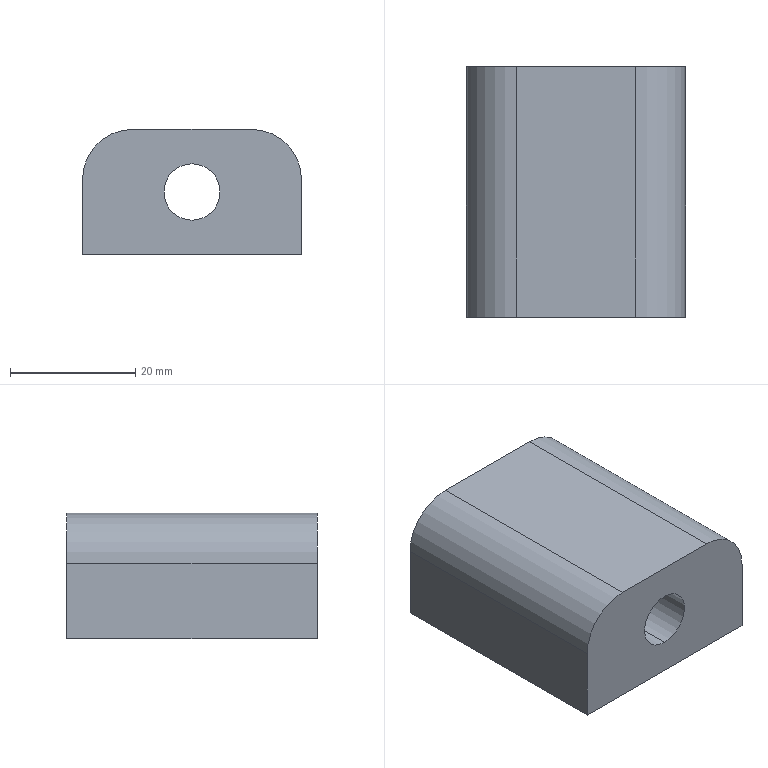Part | STEP file | 1 solid | 13 faces | box 35 x 40 x 20 mm | volume 23544 mm3 | plane 7 | cylinder 6 | commonest cylinder face diameters 9 x2 14 x2 16 x2
STEP:
#1=CARTESIAN_POINT('',(0.,0.,0.));
#2=DIRECTION('',(0.,0.,1.));
#3=DIRECTION('',(1.,0.,0.));
#4=AXIS2_PLACEMENT_3D('',#1,#2,#3);
#5=CARTESIAN_POINT('',(-72.862,-30.,211.03));
#6=VERTEX_POINT('',#5);
#7=CARTESIAN_POINT('',(-72.862,-39.,211.03));
#8=VERTEX_POINT('',#7);
#9=CARTESIAN_POINT('',(-72.862,-30.,211.03));
#10=DIRECTION('',(0.,-1.,0.));
#11=VECTOR('',#10,1.);
#12=LINE('',#9,#11);
#13=CARTESIAN_POINT('',(-72.862,-30.,218.03));
#14=DIRECTION('',(0.,-1.,0.));
#15=DIRECTION('',(0.,0.,-1.));
#16=AXIS2_PLACEMENT_3D('',#13,#14,#15);
#17=CYLINDRICAL_SURFACE('',#16,7.);
#18=CARTESIAN_POINT('',(6.283,0.));
#19=DIRECTION('',(0.,1.));
#20=VECTOR('',#19,1.);
#21=LINE('',#18,#20);
#22=(GEOMETRIC_REPRESENTATION_CONTEXT(2)PARAMETRIC_REPRESENTATION_CONTEXT()REPRESENTATION_CONTEXT('',''));
#23=DEFINITIONAL_REPRESENTATION('',(#21),#22);
#24=PCURVE('',#17,#23);
#25=CARTESIAN_POINT('',(-72.862,-30.,218.03));
#26=DIRECTION('',(0.,-1.,0.));
#27=DIRECTION('',(0.,0.,-1.));
#28=AXIS2_PLACEMENT_3D('',#25,#26,#27);
#29=CYLINDRICAL_SURFACE('',#28,7.);
#30=CARTESIAN_POINT('',(0.,0.));
#31=DIRECTION('',(0.,1.));
#32=VECTOR('',#31,1.);
#33=LINE('',#30,#32);
#34=(GEOMETRIC_REPRESENTATION_CONTEXT(2)PARAMETRIC_REPRESENTATION_CONTEXT()REPRESENTATION_CONTEXT('',''));
#35=DEFINITIONAL_REPRESENTATION('',(#33),#34);
#36=PCURVE('',#29,#35);
#37=SURFACE_CURVE('',#12,(#24,#36),.PCURVE_S1.);
#38=EDGE_CURVE('',#6,#8,#37,.T.);
#39=ORIENTED_EDGE('',*,*,#38,.T.);
#40=CARTESIAN_POINT('',(-72.862,-39.,225.03));
#41=VERTEX_POINT('',#40);
#42=CARTESIAN_POINT('',(-72.862,-39.,218.03));
#43=DIRECTION('',(0.,1.,0.));
#44=DIRECTION('',(0.,0.,1.));
#45=AXIS2_PLACEMENT_3D('',#42,#43,#44);
#46=CIRCLE('',#45,7.);
#47=CARTESIAN_POINT('',(9.425,9.));
#48=DIRECTION('',(-1.,0.));
#49=VECTOR('',#48,1.);
#50=LINE('',#47,#49);
#51=(GEOMETRIC_REPRESENTATION_CONTEXT(2)PARAMETRIC_REPRESENTATION_CONTEXT()REPRESENTATION_CONTEXT('',''));
#52=DEFINITIONAL_REPRESENTATION('',(#50),#51);
#53=PCURVE('',#17,#52);
#54=CARTESIAN_POINT('',(-72.862,-39.,218.03));
#55=DIRECTION('',(0.,-1.,0.));
#56=DIRECTION('',(0.,0.,-1.));
#57=AXIS2_PLACEMENT_3D('',#54,#55,#56);
#58=PLANE('',#57);
#59=CARTESIAN_POINT('',(-7.,0.));
#60=CARTESIAN_POINT('',(-7.,12.124));
#61=CARTESIAN_POINT('',(3.5,6.062));
#62=CARTESIAN_POINT('',(14.,0.));
#63=CARTESIAN_POINT('',(3.5,-6.062));
#64=CARTESIAN_POINT('',(-7.,-12.124));
#65=CARTESIAN_POINT('',(-7.,0.));
#66=(BOUNDED_CURVE()B_SPLINE_CURVE(2,(#59,#60,#61,#62,#63,#64,#65),.UNSPECIFIED.,.T.,.F.)B_SPLINE_CURVE_WITH_KNOTS((1,2,2,2,2,1),(-2.094,0.,2.094,4.189,6.283,8.378),.UNSPECIFIED.)CURVE()GEOMETRIC_REPRESENTATION_ITEM()RATIONAL_B_SPLINE_CURVE((1.,0.5,1.,0.5,1.,0.5,1.))REPRESENTATION_ITEM(''));
#67=(GEOMETRIC_REPRESENTATION_CONTEXT(2)PARAMETRIC_REPRESENTATION_CONTEXT()REPRESENTATION_CONTEXT('',''));
#68=DEFINITIONAL_REPRESENTATION('',(#66),#67);
#69=PCURVE('',#58,#68);
#70=SURFACE_CURVE('',#46,(#53,#69),.PCURVE_S1.);
#71=EDGE_CURVE('',#8,#41,#70,.T.);
#72=ORIENTED_EDGE('',*,*,#71,.T.);
#73=CARTESIAN_POINT('',(-72.862,-30.,225.03));
#74=VERTEX_POINT('',#73);
#75=CARTESIAN_POINT('',(-72.862,-30.,225.03));
#76=DIRECTION('',(0.,-1.,0.));
#77=VECTOR('',#76,1.);
#78=LINE('',#75,#77);
#79=CARTESIAN_POINT('',(3.142,0.));
#80=DIRECTION('',(0.,1.));
#81=VECTOR('',#80,1.);
#82=LINE('',#79,#81);
#83=(GEOMETRIC_REPRESENTATION_CONTEXT(2)PARAMETRIC_REPRESENTATION_CONTEXT()REPRESENTATION_CONTEXT('',''));
#84=DEFINITIONAL_REPRESENTATION('',(#82),#83);
#85=PCURVE('',#17,#84);
#86=CARTESIAN_POINT('',(3.142,0.));
#87=DIRECTION('',(0.,1.));
#88=VECTOR('',#87,1.);
#89=LINE('',#86,#88);
#90=(GEOMETRIC_REPRESENTATION_CONTEXT(2)PARAMETRIC_REPRESENTATION_CONTEXT()REPRESENTATION_CONTEXT('',''));
#91=DEFINITIONAL_REPRESENTATION('',(#89),#90);
#92=PCURVE('',#29,#91);
#93=SURFACE_CURVE('',#78,(#85,#92),.PCURVE_S1.);
#94=EDGE_CURVE('',#74,#41,#93,.T.);
#95=ORIENTED_EDGE('',*,*,#94,.F.);
#96=CARTESIAN_POINT('',(-72.862,-30.,218.03));
#97=DIRECTION('',(0.,-1.,0.));
#98=DIRECTION('',(0.,0.,-1.));
#99=AXIS2_PLACEMENT_3D('',#96,#97,#98);
#100=CIRCLE('',#99,7.);
#101=CARTESIAN_POINT('',(0.,0.));
#102=DIRECTION('',(1.,0.));
#103=VECTOR('',#102,1.);
#104=LINE('',#101,#103);
#105=(GEOMETRIC_REPRESENTATION_CONTEXT(2)PARAMETRIC_REPRESENTATION_CONTEXT()REPRESENTATION_CONTEXT('',''));
#106=DEFINITIONAL_REPRESENTATION('',(#104),#105);
#107=PCURVE('',#17,#106);
#108=CARTESIAN_POINT('',(-169.363,-30.,-22.97));
#109=DIRECTION('',(0.,1.,0.));
#110=DIRECTION('',(0.,0.,1.));
#111=AXIS2_PLACEMENT_3D('',#108,#109,#110);
#112=PLANE('',#111);
#113=CARTESIAN_POINT('',(234.,96.5));
#114=CARTESIAN_POINT('',(234.,108.624));
#115=CARTESIAN_POINT('',(244.5,102.562));
#116=CARTESIAN_POINT('',(255.,96.5));
#117=CARTESIAN_POINT('',(244.5,90.438));
#118=CARTESIAN_POINT('',(234.,84.376));
#119=CARTESIAN_POINT('',(234.,96.5));
#120=(BOUNDED_CURVE()B_SPLINE_CURVE(2,(#113,#114,#115,#116,#117,#118,#119),.UNSPECIFIED.,.T.,.F.)B_SPLINE_CURVE_WITH_KNOTS((1,2,2,2,2,1),(-2.094,0.,2.094,4.189,6.283,8.378),.UNSPECIFIED.)CURVE()GEOMETRIC_REPRESENTATION_ITEM()RATIONAL_B_SPLINE_CURVE((1.,0.5,1.,0.5,1.,0.5,1.))REPRESENTATION_ITEM(''));
#121=(GEOMETRIC_REPRESENTATION_CONTEXT(2)PARAMETRIC_REPRESENTATION_CONTEXT()REPRESENTATION_CONTEXT('',''));
#122=DEFINITIONAL_REPRESENTATION('',(#120),#121);
#123=PCURVE('',#112,#122);
#124=SURFACE_CURVE('',#100,(#107,#123),.PCURVE_S1.);
#125=EDGE_CURVE('',#74,#6,#124,.T.);
#126=ORIENTED_EDGE('',*,*,#125,.T.);
#127=EDGE_LOOP('',(#39,#72,#95,#126));
#128=FACE_BOUND('',#127,.F.);
#129=ADVANCED_FACE('',(#128),#17,.F.);
#130=CARTESIAN_POINT('',(-72.862,-39.,213.53));
#131=VERTEX_POINT('',#130);
#132=CARTESIAN_POINT('',(-72.862,-70.,213.53));
#133=VERTEX_POINT('',#132);
#134=CARTESIAN_POINT('',(-72.862,-30.,213.53));
#135=DIRECTION('',(0.,-1.,0.));
#136=VECTOR('',#135,1.);
#137=LINE('',#134,#136);
#138=CARTESIAN_POINT('',(-72.862,-30.,218.03));
#139=DIRECTION('',(0.,-1.,0.));
#140=DIRECTION('',(0.,0.,-1.));
#141=AXIS2_PLACEMENT_3D('',#138,#139,#140);
#142=CYLINDRICAL_SURFACE('',#141,4.5);
#143=CARTESIAN_POINT('',(6.283,0.));
#144=DIRECTION('',(0.,1.));
#145=VECTOR('',#144,1.);
#146=LINE('',#143,#145);
#147=(GEOMETRIC_REPRESENTATION_CONTEXT(2)PARAMETRIC_REPRESENTATION_CONTEXT()REPRESENTATION_CONTEXT('',''));
#148=DEFINITIONAL_REPRESENTATION('',(#146),#147);
#149=PCURVE('',#142,#148);
#150=CARTESIAN_POINT('',(-72.862,-30.,218.03));
#151=DIRECTION('',(0.,-1.,0.));
#152=DIRECTION('',(0.,0.,-1.));
#153=AXIS2_PLACEMENT_3D('',#150,#151,#152);
#154=CYLINDRICAL_SURFACE('',#153,4.5);
#155=CARTESIAN_POINT('',(0.,0.));
#156=DIRECTION('',(0.,1.));
#157=VECTOR('',#156,1.);
#158=LINE('',#155,#157);
#159=(GEOMETRIC_REPRESENTATION_CONTEXT(2)PARAMETRIC_REPRESENTATION_CONTEXT()REPRESENTATION_CONTEXT('',''));
#160=DEFINITIONAL_REPRESENTATION('',(#158),#159);
#161=PCURVE('',#154,#160);
#162=SURFACE_CURVE('',#137,(#149,#161),.PCURVE_S1.);
#163=EDGE_CURVE('',#131,#133,#162,.T.);
#164=ORIENTED_EDGE('',*,*,#163,.T.);
#165=CARTESIAN_POINT('',(-72.862,-70.,222.53));
#166=VERTEX_POINT('',#165);
#167=CARTESIAN_POINT('',(-72.862,-70.,218.03));
#168=DIRECTION('',(0.,1.,0.));
#169=DIRECTION('',(0.,0.,1.));
#170=AXIS2_PLACEMENT_3D('',#167,#168,#169);
#171=CIRCLE('',#170,4.5);
#172=CARTESIAN_POINT('',(9.425,40.));
#173=DIRECTION('',(-1.,0.));
#174=VECTOR('',#173,1.);
#175=LINE('',#172,#174);
#176=(GEOMETRIC_REPRESENTATION_CONTEXT(2)PARAMETRIC_REPRESENTATION_CONTEXT()REPRESENTATION_CONTEXT('',''));
#177=DEFINITIONAL_REPRESENTATION('',(#175),#176);
#178=PCURVE('',#142,#177);
#179=CARTESIAN_POINT('',(-72.862,-70.,23.556));
#180=DIRECTION('',(0.,-1.,0.));
#181=DIRECTION('',(0.,0.,-1.));
#182=AXIS2_PLACEMENT_3D('',#179,#180,#181);
#183=PLANE('',#182);
#184=CARTESIAN_POINT('',(-198.974,0.));
#185=CARTESIAN_POINT('',(-198.974,7.794));
#186=CARTESIAN_POINT('',(-192.224,3.897));
#187=CARTESIAN_POINT('',(-185.474,0.));
#188=CARTESIAN_POINT('',(-192.224,-3.897));
#189=CARTESIAN_POINT('',(-198.974,-7.794));
#190=CARTESIAN_POINT('',(-198.974,0.));
#191=(BOUNDED_CURVE()B_SPLINE_CURVE(2,(#184,#185,#186,#187,#188,#189,#190),.UNSPECIFIED.,.T.,.F.)B_SPLINE_CURVE_WITH_KNOTS((1,2,2,2,2,1),(-2.094,0.,2.094,4.189,6.283,8.378),.UNSPECIFIED.)CURVE()GEOMETRIC_REPRESENTATION_ITEM()RATIONAL_B_SPLINE_CURVE((1.,0.5,1.,0.5,1.,0.5,1.))REPRESENTATION_ITEM(''));
#192=(GEOMETRIC_REPRESENTATION_CONTEXT(2)PARAMETRIC_REPRESENTATION_CONTEXT()REPRESENTATION_CONTEXT('',''));
#193=DEFINITIONAL_REPRESENTATION('',(#191),#192);
#194=PCURVE('',#183,#193);
#195=SURFACE_CURVE('',#171,(#178,#194),.PCURVE_S1.);
#196=EDGE_CURVE('',#133,#166,#195,.T.);
#197=ORIENTED_EDGE('',*,*,#196,.T.);
#198=CARTESIAN_POINT('',(-72.862,-39.,222.53));
#199=VERTEX_POINT('',#198);
#200=CARTESIAN_POINT('',(-72.862,-30.,222.53));
#201=DIRECTION('',(0.,-1.,0.));
#202=VECTOR('',#201,1.);
#203=LINE('',#200,#202);
#204=CARTESIAN_POINT('',(3.142,0.));
#205=DIRECTION('',(0.,1.));
#206=VECTOR('',#205,1.);
#207=LINE('',#204,#206);
#208=(GEOMETRIC_REPRESENTATION_CONTEXT(2)PARAMETRIC_REPRESENTATION_CONTEXT()REPRESENTATION_CONTEXT('',''));
#209=DEFINITIONAL_REPRESENTATION('',(#207),#208);
#210=PCURVE('',#142,#209);
#211=CARTESIAN_POINT('',(3.142,0.));
#212=DIRECTION('',(0.,1.));
#213=VECTOR('',#212,1.);
#214=LINE('',#211,#213);
#215=(GEOMETRIC_REPRESENTATION_CONTEXT(2)PARAMETRIC_REPRESENTATION_CONTEXT()REPRESENTATION_CONTEXT('',''));
#216=DEFINITIONAL_REPRESENTATION('',(#214),#215);
#217=PCURVE('',#154,#216);
#218=SURFACE_CURVE('',#203,(#210,#217),.PCURVE_S1.);
#219=EDGE_CURVE('',#199,#166,#218,.T.);
#220=ORIENTED_EDGE('',*,*,#219,.F.);
#221=CARTESIAN_POINT('',(-72.862,-39.,218.03));
#222=DIRECTION('',(0.,1.,0.));
#223=DIRECTION('',(0.,0.,-1.));
#224=AXIS2_PLACEMENT_3D('',#221,#222,#223);
#225=CIRCLE('',#224,4.5);
#226=CARTESIAN_POINT('',(6.283,9.));
#227=DIRECTION('',(-1.,0.));
#228=VECTOR('',#227,1.);
#229=LINE('',#226,#228);
#230=(GEOMETRIC_REPRESENTATION_CONTEXT(2)PARAMETRIC_REPRESENTATION_CONTEXT()REPRESENTATION_CONTEXT('',''));
#231=DEFINITIONAL_REPRESENTATION('',(#229),#230);
#232=PCURVE('',#142,#231);
#233=CARTESIAN_POINT('',(4.5,0.));
#234=CARTESIAN_POINT('',(4.5,-7.794));
#235=CARTESIAN_POINT('',(-2.25,-3.897));
#236=CARTESIAN_POINT('',(-9.,0.));
#237=CARTESIAN_POINT('',(-2.25,3.897));
#238=CARTESIAN_POINT('',(4.5,7.794));
#239=CARTESIAN_POINT('',(4.5,0.));
#240=(BOUNDED_CURVE()B_SPLINE_CURVE(2,(#233,#234,#235,#236,#237,#238,#239),.UNSPECIFIED.,.T.,.F.)B_SPLINE_CURVE_WITH_KNOTS((1,2,2,2,2,1),(-2.094,0.,2.094,4.189,6.283,8.378),.UNSPECIFIED.)CURVE()GEOMETRIC_REPRESENTATION_ITEM()RATIONAL_B_SPLINE_CURVE((1.,0.5,1.,0.5,1.,0.5,1.))REPRESENTATION_ITEM(''));
#241=(GEOMETRIC_REPRESENTATION_CONTEXT(2)PARAMETRIC_REPRESENTATION_CONTEXT()REPRESENTATION_CONTEXT('',''));
#242=DEFINITIONAL_REPRESENTATION('',(#240),#241);
#243=PCURVE('',#58,#242);
#244=SURFACE_CURVE('',#225,(#232,#243),.PCURVE_S1.);
#245=EDGE_CURVE('',#131,#199,#244,.T.);
#246=ORIENTED_EDGE('',*,*,#245,.F.);
#247=EDGE_LOOP('',(#164,#197,#220,#246));
#248=FACE_BOUND('',#247,.F.);
#249=ADVANCED_FACE('',(#248),#142,.F.);
#250=CARTESIAN_POINT('',(-90.362,-70.,220.03));
#251=VERTEX_POINT('',#250);
#252=CARTESIAN_POINT('',(-82.362,-70.,228.03));
#253=VERTEX_POINT('',#252);
#254=CARTESIAN_POINT('',(-82.362,-70.,220.03));
#255=DIRECTION('',(0.,1.,0.));
#256=DIRECTION('',(0.,0.,-1.));
#257=AXIS2_PLACEMENT_3D('',#254,#255,#256);
#258=CIRCLE('',#257,8.);
#259=CARTESIAN_POINT('',(-188.474,-9.5));
#260=CARTESIAN_POINT('',(-188.474,-23.356));
#261=CARTESIAN_POINT('',(-200.474,-16.428));
#262=CARTESIAN_POINT('',(-212.474,-9.5));
#263=CARTESIAN_POINT('',(-200.474,-2.572));
#264=CARTESIAN_POINT('',(-188.474,4.356));
#265=CARTESIAN_POINT('',(-188.474,-9.5));
#266=(BOUNDED_CURVE()B_SPLINE_CURVE(2,(#259,#260,#261,#262,#263,#264,#265),.UNSPECIFIED.,.T.,.F.)B_SPLINE_CURVE_WITH_KNOTS((1,2,2,2,2,1),(-2.094,0.,2.094,4.189,6.283,8.378),.UNSPECIFIED.)CURVE()GEOMETRIC_REPRESENTATION_ITEM()RATIONAL_B_SPLINE_CURVE((1.,0.5,1.,0.5,1.,0.5,1.))REPRESENTATION_ITEM(''));
#267=(GEOMETRIC_REPRESENTATION_CONTEXT(2)PARAMETRIC_REPRESENTATION_CONTEXT()REPRESENTATION_CONTEXT('',''));
#268=DEFINITIONAL_REPRESENTATION('',(#266),#267);
#269=PCURVE('',#183,#268);
#270=CARTESIAN_POINT('',(-82.362,-85.,220.03));
#271=DIRECTION('',(0.,1.,0.));
#272=DIRECTION('',(0.,0.,1.));
#273=AXIS2_PLACEMENT_3D('',#270,#271,#272);
#274=CYLINDRICAL_SURFACE('',#273,8.);
#275=CARTESIAN_POINT('',(3.142,15.));
#276=DIRECTION('',(1.,0.));
#277=VECTOR('',#276,1.);
#278=LINE('',#275,#277);
#279=(GEOMETRIC_REPRESENTATION_CONTEXT(2)PARAMETRIC_REPRESENTATION_CONTEXT()REPRESENTATION_CONTEXT('',''));
#280=DEFINITIONAL_REPRESENTATION('',(#278),#279);
#281=PCURVE('',#274,#280);
#282=SURFACE_CURVE('',#258,(#269,#281),.PCURVE_S1.);
#283=EDGE_CURVE('',#251,#253,#282,.T.);
#284=ORIENTED_EDGE('',*,*,#283,.F.);
#285=CARTESIAN_POINT('',(-90.362,-70.,208.03));
#286=VERTEX_POINT('',#285);
#287=CARTESIAN_POINT('',(-90.362,-70.,155.78));
#288=DIRECTION('',(0.,0.,1.));
#289=VECTOR('',#288,1.);
#290=LINE('',#287,#289);
#291=CARTESIAN_POINT('',(-132.224,-17.5));
#292=DIRECTION('',(-1.,0.));
#293=VECTOR('',#292,1.);
#294=LINE('',#291,#293);
#295=(GEOMETRIC_REPRESENTATION_CONTEXT(2)PARAMETRIC_REPRESENTATION_CONTEXT()REPRESENTATION_CONTEXT('',''));
#296=DEFINITIONAL_REPRESENTATION('',(#294),#295);
#297=PCURVE('',#183,#296);
#298=CARTESIAN_POINT('',(-90.362,-85.,155.78));
#299=DIRECTION('',(-1.,0.,0.));
#300=DIRECTION('',(0.,0.,1.));
#301=AXIS2_PLACEMENT_3D('',#298,#299,#300);
#302=PLANE('',#301);
#303=CARTESIAN_POINT('',(0.,15.));
#304=DIRECTION('',(1.,0.));
#305=VECTOR('',#304,1.);
#306=LINE('',#303,#305);
#307=(GEOMETRIC_REPRESENTATION_CONTEXT(2)PARAMETRIC_REPRESENTATION_CONTEXT()REPRESENTATION_CONTEXT('',''));
#308=DEFINITIONAL_REPRESENTATION('',(#306),#307);
#309=PCURVE('',#302,#308);
#310=SURFACE_CURVE('',#290,(#297,#309),.PCURVE_S1.);
#311=EDGE_CURVE('',#286,#251,#310,.T.);
#312=ORIENTED_EDGE('',*,*,#311,.F.);
#313=CARTESIAN_POINT('',(-55.362,-70.,208.03));
#314=VERTEX_POINT('',#313);
#315=CARTESIAN_POINT('',(-72.862,-70.,208.03));
#316=DIRECTION('',(1.,0.,0.));
#317=VECTOR('',#316,1.);
#318=LINE('',#315,#317);
#319=CARTESIAN_POINT('',(-184.474,0.));
#320=DIRECTION('',(0.,1.));
#321=VECTOR('',#320,1.);
#322=LINE('',#319,#321);
#323=(GEOMETRIC_REPRESENTATION_CONTEXT(2)PARAMETRIC_REPRESENTATION_CONTEXT()REPRESENTATION_CONTEXT('',''));
#324=DEFINITIONAL_REPRESENTATION('',(#322),#323);
#325=PCURVE('',#183,#324);
#326=CARTESIAN_POINT('',(-72.862,-40.,208.03));
#327=DIRECTION('',(0.,0.,1.));
#328=DIRECTION('',(1.,0.,0.));
#329=AXIS2_PLACEMENT_3D('',#326,#327,#328);
#330=PLANE('',#329);
#331=CARTESIAN_POINT('',(0.,-30.));
#332=DIRECTION('',(1.,0.));
#333=VECTOR('',#332,1.);
#334=LINE('',#331,#333);
#335=(GEOMETRIC_REPRESENTATION_CONTEXT(2)PARAMETRIC_REPRESENTATION_CONTEXT()REPRESENTATION_CONTEXT('',''));
#336=DEFINITIONAL_REPRESENTATION('',(#334),#335);
#337=PCURVE('',#330,#336);
#338=SURFACE_CURVE('',#318,(#325,#337),.PCURVE_S1.);
#339=EDGE_CURVE('',#286,#314,#338,.T.);
#340=ORIENTED_EDGE('',*,*,#339,.T.);
#341=CARTESIAN_POINT('',(-55.362,-70.,220.03));
#342=VERTEX_POINT('',#341);
#343=CARTESIAN_POINT('',(-55.362,-70.,23.556));
#344=DIRECTION('',(0.,0.,1.));
#345=VECTOR('',#344,1.);
#346=LINE('',#343,#345);
#347=CARTESIAN_POINT('',(0.,17.5));
#348=DIRECTION('',(-1.,0.));
#349=VECTOR('',#348,1.);
#350=LINE('',#347,#349);
#351=(GEOMETRIC_REPRESENTATION_CONTEXT(2)PARAMETRIC_REPRESENTATION_CONTEXT()REPRESENTATION_CONTEXT('',''));
#352=DEFINITIONAL_REPRESENTATION('',(#350),#351);
#353=PCURVE('',#183,#352);
#354=CARTESIAN_POINT('',(-55.362,-85.,155.78));
#355=DIRECTION('',(1.,0.,0.));
#356=DIRECTION('',(0.,0.,-1.));
#357=AXIS2_PLACEMENT_3D('',#354,#355,#356);
#358=PLANE('',#357);
#359=CARTESIAN_POINT('',(132.224,15.));
#360=DIRECTION('',(-1.,0.));
#361=VECTOR('',#360,1.);
#362=LINE('',#359,#361);
#363=(GEOMETRIC_REPRESENTATION_CONTEXT(2)PARAMETRIC_REPRESENTATION_CONTEXT()REPRESENTATION_CONTEXT('',''));
#364=DEFINITIONAL_REPRESENTATION('',(#362),#363);
#365=PCURVE('',#358,#364);
#366=SURFACE_CURVE('',#346,(#353,#365),.PCURVE_S1.);
#367=EDGE_CURVE('',#314,#342,#366,.T.);
#368=ORIENTED_EDGE('',*,*,#367,.T.);
#369=CARTESIAN_POINT('',(-63.362,-70.,228.03));
#370=VERTEX_POINT('',#369);
#371=CARTESIAN_POINT('',(-63.362,-70.,220.03));
#372=DIRECTION('',(0.,1.,0.));
#373=DIRECTION('',(0.,0.,-1.));
#374=AXIS2_PLACEMENT_3D('',#371,#372,#373);
#375=CIRCLE('',#374,8.);
#376=CARTESIAN_POINT('',(-188.474,9.5));
#377=CARTESIAN_POINT('',(-188.474,-4.356));
#378=CARTESIAN_POINT('',(-200.474,2.572));
#379=CARTESIAN_POINT('',(-212.474,9.5));
#380=CARTESIAN_POINT('',(-200.474,16.428));
#381=CARTESIAN_POINT('',(-188.474,23.356));
#382=CARTESIAN_POINT('',(-188.474,9.5));
#383=(BOUNDED_CURVE()B_SPLINE_CURVE(2,(#376,#377,#378,#379,#380,#381,#382),.UNSPECIFIED.,.T.,.F.)B_SPLINE_CURVE_WITH_KNOTS((1,2,2,2,2,1),(-2.094,0.,2.094,4.189,6.283,8.378),.UNSPECIFIED.)CURVE()GEOMETRIC_REPRESENTATION_ITEM()RATIONAL_B_SPLINE_CURVE((1.,0.5,1.,0.5,1.,0.5,1.))REPRESENTATION_ITEM(''));
#384=(GEOMETRIC_REPRESENTATION_CONTEXT(2)PARAMETRIC_REPRESENTATION_CONTEXT()REPRESENTATION_CONTEXT('',''));
#385=DEFINITIONAL_REPRESENTATION('',(#383),#384);
#386=PCURVE('',#183,#385);
#387=CARTESIAN_POINT('',(-63.362,-40.,220.03));
#388=DIRECTION('',(0.,1.,0.));
#389=DIRECTION('',(0.,0.,1.));
#390=AXIS2_PLACEMENT_3D('',#387,#388,#389);
#391=CYLINDRICAL_SURFACE('',#390,8.);
#392=CARTESIAN_POINT('',(-3.142,-30.));
#393=DIRECTION('',(1.,0.));
#394=VECTOR('',#393,1.);
#395=LINE('',#392,#394);
#396=(GEOMETRIC_REPRESENTATION_CONTEXT(2)PARAMETRIC_REPRESENTATION_CONTEXT()REPRESENTATION_CONTEXT('',''));
#397=DEFINITIONAL_REPRESENTATION('',(#395),#396);
#398=PCURVE('',#391,#397);
#399=SURFACE_CURVE('',#375,(#386,#398),.PCURVE_S1.);
#400=EDGE_CURVE('',#370,#342,#399,.T.);
#401=ORIENTED_EDGE('',*,*,#400,.F.);
#402=CARTESIAN_POINT('',(-72.862,-70.,228.03));
#403=DIRECTION('',(-1.,0.,0.));
#404=VECTOR('',#403,1.);
#405=LINE('',#402,#404);
#406=CARTESIAN_POINT('',(-204.474,0.));
#407=DIRECTION('',(0.,-1.));
#408=VECTOR('',#407,1.);
#409=LINE('',#406,#408);
#410=(GEOMETRIC_REPRESENTATION_CONTEXT(2)PARAMETRIC_REPRESENTATION_CONTEXT()REPRESENTATION_CONTEXT('',''));
#411=DEFINITIONAL_REPRESENTATION('',(#409),#410);
#412=PCURVE('',#183,#411);
#413=CARTESIAN_POINT('',(-72.862,-40.,228.03));
#414=DIRECTION('',(0.,0.,1.));
#415=DIRECTION('',(1.,0.,0.));
#416=AXIS2_PLACEMENT_3D('',#413,#414,#415);
#417=PLANE('',#416);
#418=CARTESIAN_POINT('',(0.,-30.));
#419=DIRECTION('',(-1.,0.));
#420=VECTOR('',#419,1.);
#421=LINE('',#418,#420);
#422=(GEOMETRIC_REPRESENTATION_CONTEXT(2)PARAMETRIC_REPRESENTATION_CONTEXT()REPRESENTATION_CONTEXT('',''));
#423=DEFINITIONAL_REPRESENTATION('',(#421),#422);
#424=PCURVE('',#417,#423);
#425=SURFACE_CURVE('',#405,(#412,#424),.PCURVE_S1.);
#426=EDGE_CURVE('',#370,#253,#425,.T.);
#427=ORIENTED_EDGE('',*,*,#426,.T.);
#428=EDGE_LOOP('',(#284,#312,#340,#368,#401,#427));
#429=FACE_BOUND('',#428,.T.);
#430=ORIENTED_EDGE('',*,*,#196,.T.);
#431=CARTESIAN_POINT('',(-72.862,-70.,218.03));
#432=DIRECTION('',(0.,1.,0.));
#433=DIRECTION('',(0.,0.,1.));
#434=AXIS2_PLACEMENT_3D('',#431,#432,#433);
#435=CIRCLE('',#434,4.5);
#436=CARTESIAN_POINT('',(-198.974,0.));
#437=CARTESIAN_POINT('',(-198.974,7.794));
#438=CARTESIAN_POINT('',(-192.224,3.897));
#439=CARTESIAN_POINT('',(-185.474,0.));
#440=CARTESIAN_POINT('',(-192.224,-3.897));
#441=CARTESIAN_POINT('',(-198.974,-7.794));
#442=CARTESIAN_POINT('',(-198.974,0.));
#443=(BOUNDED_CURVE()B_SPLINE_CURVE(2,(#436,#437,#438,#439,#440,#441,#442),.UNSPECIFIED.,.T.,.F.)B_SPLINE_CURVE_WITH_KNOTS((1,2,2,2,2,1),(-2.094,0.,2.094,4.189,6.283,8.378),.UNSPECIFIED.)CURVE()GEOMETRIC_REPRESENTATION_ITEM()RATIONAL_B_SPLINE_CURVE((1.,0.5,1.,0.5,1.,0.5,1.))REPRESENTATION_ITEM(''));
#444=(GEOMETRIC_REPRESENTATION_CONTEXT(2)PARAMETRIC_REPRESENTATION_CONTEXT()REPRESENTATION_CONTEXT('',''));
#445=DEFINITIONAL_REPRESENTATION('',(#443),#444);
#446=PCURVE('',#183,#445);
#447=CARTESIAN_POINT('',(3.142,40.));
#448=DIRECTION('',(-1.,0.));
#449=VECTOR('',#448,1.);
#450=LINE('',#447,#449);
#451=(GEOMETRIC_REPRESENTATION_CONTEXT(2)PARAMETRIC_REPRESENTATION_CONTEXT()REPRESENTATION_CONTEXT('',''));
#452=DEFINITIONAL_REPRESENTATION('',(#450),#451);
#453=PCURVE('',#154,#452);
#454=SURFACE_CURVE('',#435,(#446,#453),.PCURVE_S1.);
#455=EDGE_CURVE('',#166,#133,#454,.T.);
#456=ORIENTED_EDGE('',*,*,#455,.T.);
#457=EDGE_LOOP('',(#430,#456));
#458=FACE_BOUND('',#457,.T.);
#459=ADVANCED_FACE('',(#429,#458),#183,.T.);
#460=CARTESIAN_POINT('',(-72.862,-30.,218.03));
#461=DIRECTION('',(0.,-1.,0.));
#462=DIRECTION('',(0.,0.,-1.));
#463=AXIS2_PLACEMENT_3D('',#460,#461,#462);
#464=CIRCLE('',#463,7.);
#465=CARTESIAN_POINT('',(234.,96.5));
#466=CARTESIAN_POINT('',(234.,108.624));
#467=CARTESIAN_POINT('',(244.5,102.562));
#468=CARTESIAN_POINT('',(255.,96.5));
#469=CARTESIAN_POINT('',(244.5,90.438));
#470=CARTESIAN_POINT('',(234.,84.376));
#471=CARTESIAN_POINT('',(234.,96.5));
#472=(BOUNDED_CURVE()B_SPLINE_CURVE(2,(#465,#466,#467,#468,#469,#470,#471),.UNSPECIFIED.,.T.,.F.)B_SPLINE_CURVE_WITH_KNOTS((1,2,2,2,2,1),(-2.094,0.,2.094,4.189,6.283,8.378),.UNSPECIFIED.)CURVE()GEOMETRIC_REPRESENTATION_ITEM()RATIONAL_B_SPLINE_CURVE((1.,0.5,1.,0.5,1.,0.5,1.))REPRESENTATION_ITEM(''));
#473=(GEOMETRIC_REPRESENTATION_CONTEXT(2)PARAMETRIC_REPRESENTATION_CONTEXT()REPRESENTATION_CONTEXT('',''));
#474=DEFINITIONAL_REPRESENTATION('',(#472),#473);
#475=PCURVE('',#112,#474);
#476=CARTESIAN_POINT('',(0.,0.));
#477=DIRECTION('',(1.,0.));
#478=VECTOR('',#477,1.);
#479=LINE('',#476,#478);
#480=(GEOMETRIC_REPRESENTATION_CONTEXT(2)PARAMETRIC_REPRESENTATION_CONTEXT()REPRESENTATION_CONTEXT('',''));
#481=DEFINITIONAL_REPRESENTATION('',(#479),#480);
#482=PCURVE('',#29,#481);
#483=SURFACE_CURVE('',#464,(#475,#482),.PCURVE_S1.);
#484=EDGE_CURVE('',#6,#74,#483,.T.);
#485=ORIENTED_EDGE('',*,*,#484,.T.);
#486=ORIENTED_EDGE('',*,*,#125,.T.);
#487=EDGE_LOOP('',(#485,#486));
#488=FACE_BOUND('',#487,.T.);
#489=CARTESIAN_POINT('',(-55.362,-30.,220.03));
#490=VERTEX_POINT('',#489);
#491=CARTESIAN_POINT('',(-63.362,-30.,228.03));
#492=VERTEX_POINT('',#491);
#493=CARTESIAN_POINT('',(-63.362,-30.,220.03));
#494=DIRECTION('',(0.,-1.,0.));
#495=DIRECTION('',(0.,0.,1.));
#496=AXIS2_PLACEMENT_3D('',#493,#494,#495);
#497=CIRCLE('',#496,8.);
#498=CARTESIAN_POINT('',(251.,106.));
#499=CARTESIAN_POINT('',(251.,92.144));
#500=CARTESIAN_POINT('',(239.,99.072));
#501=CARTESIAN_POINT('',(227.,106.));
#502=CARTESIAN_POINT('',(239.,112.928));
#503=CARTESIAN_POINT('',(251.,119.856));
#504=CARTESIAN_POINT('',(251.,106.));
#505=(BOUNDED_CURVE()B_SPLINE_CURVE(2,(#498,#499,#500,#501,#502,#503,#504),.UNSPECIFIED.,.T.,.F.)B_SPLINE_CURVE_WITH_KNOTS((1,2,2,2,2,1),(-2.094,0.,2.094,4.189,6.283,8.378),.UNSPECIFIED.)CURVE()GEOMETRIC_REPRESENTATION_ITEM()RATIONAL_B_SPLINE_CURVE((1.,0.5,1.,0.5,1.,0.5,1.))REPRESENTATION_ITEM(''));
#506=(GEOMETRIC_REPRESENTATION_CONTEXT(2)PARAMETRIC_REPRESENTATION_CONTEXT()REPRESENTATION_CONTEXT('',''));
#507=DEFINITIONAL_REPRESENTATION('',(#505),#506);
#508=PCURVE('',#112,#507);
#509=CARTESIAN_POINT('',(6.283,10.));
#510=DIRECTION('',(-1.,0.));
#511=VECTOR('',#510,1.);
#512=LINE('',#509,#511);
#513=(GEOMETRIC_REPRESENTATION_CONTEXT(2)PARAMETRIC_REPRESENTATION_CONTEXT()REPRESENTATION_CONTEXT('',''));
#514=DEFINITIONAL_REPRESENTATION('',(#512),#513);
#515=PCURVE('',#391,#514);
#516=SURFACE_CURVE('',#497,(#508,#515),.PCURVE_S1.);
#517=EDGE_CURVE('',#490,#492,#516,.T.);
#518=ORIENTED_EDGE('',*,*,#517,.F.);
#519=CARTESIAN_POINT('',(-55.362,-30.,208.03));
#520=VERTEX_POINT('',#519);
#521=CARTESIAN_POINT('',(-55.362,-30.,155.78));
#522=DIRECTION('',(0.,0.,1.));
#523=VECTOR('',#522,1.);
#524=LINE('',#521,#523);
#525=CARTESIAN_POINT('',(178.75,114.));
#526=DIRECTION('',(1.,0.));
#527=VECTOR('',#526,1.);
#528=LINE('',#525,#527);
#529=(GEOMETRIC_REPRESENTATION_CONTEXT(2)PARAMETRIC_REPRESENTATION_CONTEXT()REPRESENTATION_CONTEXT('',''));
#530=DEFINITIONAL_REPRESENTATION('',(#528),#529);
#531=PCURVE('',#112,#530);
#532=CARTESIAN_POINT('',(0.,55.));
#533=DIRECTION('',(-1.,0.));
#534=VECTOR('',#533,1.);
#535=LINE('',#532,#534);
#536=(GEOMETRIC_REPRESENTATION_CONTEXT(2)PARAMETRIC_REPRESENTATION_CONTEXT()REPRESENTATION_CONTEXT('',''));
#537=DEFINITIONAL_REPRESENTATION('',(#535),#536);
#538=PCURVE('',#358,#537);
#539=SURFACE_CURVE('',#524,(#531,#538),.PCURVE_S1.);
#540=EDGE_CURVE('',#520,#490,#539,.T.);
#541=ORIENTED_EDGE('',*,*,#540,.F.);
#542=CARTESIAN_POINT('',(-90.362,-30.,208.03));
#543=VERTEX_POINT('',#542);
#544=CARTESIAN_POINT('',(-169.363,-30.,208.03));
#545=DIRECTION('',(-1.,0.,0.));
#546=VECTOR('',#545,1.);
#547=LINE('',#544,#546);
#548=CARTESIAN_POINT('',(231.,0.));
#549=DIRECTION('',(0.,-1.));
#550=VECTOR('',#549,1.);
#551=LINE('',#548,#550);
#552=(GEOMETRIC_REPRESENTATION_CONTEXT(2)PARAMETRIC_REPRESENTATION_CONTEXT()REPRESENTATION_CONTEXT('',''));
#553=DEFINITIONAL_REPRESENTATION('',(#551),#552);
#554=PCURVE('',#112,#553);
#555=CARTESIAN_POINT('',(-96.5,10.));
#556=DIRECTION('',(-1.,0.));
#557=VECTOR('',#556,1.);
#558=LINE('',#555,#557);
#559=(GEOMETRIC_REPRESENTATION_CONTEXT(2)PARAMETRIC_REPRESENTATION_CONTEXT()REPRESENTATION_CONTEXT('',''));
#560=DEFINITIONAL_REPRESENTATION('',(#558),#559);
#561=PCURVE('',#330,#560);
#562=SURFACE_CURVE('',#547,(#554,#561),.PCURVE_S1.);
#563=EDGE_CURVE('',#520,#543,#562,.T.);
#564=ORIENTED_EDGE('',*,*,#563,.T.);
#565=CARTESIAN_POINT('',(-90.362,-30.,220.03));
#566=VERTEX_POINT('',#565);
#567=CARTESIAN_POINT('',(-90.362,-30.,-22.97));
#568=DIRECTION('',(0.,0.,1.));
#569=VECTOR('',#568,1.);
#570=LINE('',#567,#569);
#571=CARTESIAN_POINT('',(0.,79.));
#572=DIRECTION('',(1.,0.));
#573=VECTOR('',#572,1.);
#574=LINE('',#571,#573);
#575=(GEOMETRIC_REPRESENTATION_CONTEXT(2)PARAMETRIC_REPRESENTATION_CONTEXT()REPRESENTATION_CONTEXT('',''));
#576=DEFINITIONAL_REPRESENTATION('',(#574),#575);
#577=PCURVE('',#112,#576);
#578=CARTESIAN_POINT('',(-178.75,55.));
#579=DIRECTION('',(1.,0.));
#580=VECTOR('',#579,1.);
#581=LINE('',#578,#580);
#582=(GEOMETRIC_REPRESENTATION_CONTEXT(2)PARAMETRIC_REPRESENTATION_CONTEXT()REPRESENTATION_CONTEXT('',''));
#583=DEFINITIONAL_REPRESENTATION('',(#581),#582);
#584=PCURVE('',#302,#583);
#585=SURFACE_CURVE('',#570,(#577,#584),.PCURVE_S1.);
#586=EDGE_CURVE('',#543,#566,#585,.T.);
#587=ORIENTED_EDGE('',*,*,#586,.T.);
#588=CARTESIAN_POINT('',(-82.362,-30.,228.03));
#589=VERTEX_POINT('',#588);
#590=CARTESIAN_POINT('',(-82.362,-30.,220.03));
#591=DIRECTION('',(0.,-1.,0.));
#592=DIRECTION('',(0.,0.,1.));
#593=AXIS2_PLACEMENT_3D('',#590,#591,#592);
#594=CIRCLE('',#593,8.);
#595=CARTESIAN_POINT('',(251.,87.));
#596=CARTESIAN_POINT('',(251.,73.144));
#597=CARTESIAN_POINT('',(239.,80.072));
#598=CARTESIAN_POINT('',(227.,87.));
#599=CARTESIAN_POINT('',(239.,93.928));
#600=CARTESIAN_POINT('',(251.,100.856));
#601=CARTESIAN_POINT('',(251.,87.));
#602=(BOUNDED_CURVE()B_SPLINE_CURVE(2,(#595,#596,#597,#598,#599,#600,#601),.UNSPECIFIED.,.T.,.F.)B_SPLINE_CURVE_WITH_KNOTS((1,2,2,2,2,1),(-2.094,0.,2.094,4.189,6.283,8.378),.UNSPECIFIED.)CURVE()GEOMETRIC_REPRESENTATION_ITEM()RATIONAL_B_SPLINE_CURVE((1.,0.5,1.,0.5,1.,0.5,1.))REPRESENTATION_ITEM(''));
#603=(GEOMETRIC_REPRESENTATION_CONTEXT(2)PARAMETRIC_REPRESENTATION_CONTEXT()REPRESENTATION_CONTEXT('',''));
#604=DEFINITIONAL_REPRESENTATION('',(#602),#603);
#605=PCURVE('',#112,#604);
#606=CARTESIAN_POINT('',(6.283,55.));
#607=DIRECTION('',(-1.,0.));
#608=VECTOR('',#607,1.);
#609=LINE('',#606,#608);
#610=(GEOMETRIC_REPRESENTATION_CONTEXT(2)PARAMETRIC_REPRESENTATION_CONTEXT()REPRESENTATION_CONTEXT('',''));
#611=DEFINITIONAL_REPRESENTATION('',(#609),#610);
#612=PCURVE('',#274,#611);
#613=SURFACE_CURVE('',#594,(#605,#612),.PCURVE_S1.);
#614=EDGE_CURVE('',#589,#566,#613,.T.);
#615=ORIENTED_EDGE('',*,*,#614,.F.);
#616=CARTESIAN_POINT('',(-169.363,-30.,228.03));
#617=DIRECTION('',(1.,0.,0.));
#618=VECTOR('',#617,1.);
#619=LINE('',#616,#618);
#620=CARTESIAN_POINT('',(251.,0.));
#621=DIRECTION('',(0.,1.));
#622=VECTOR('',#621,1.);
#623=LINE('',#620,#622);
#624=(GEOMETRIC_REPRESENTATION_CONTEXT(2)PARAMETRIC_REPRESENTATION_CONTEXT()REPRESENTATION_CONTEXT('',''));
#625=DEFINITIONAL_REPRESENTATION('',(#623),#624);
#626=PCURVE('',#112,#625);
#627=CARTESIAN_POINT('',(-96.5,10.));
#628=DIRECTION('',(1.,0.));
#629=VECTOR('',#628,1.);
#630=LINE('',#627,#629);
#631=(GEOMETRIC_REPRESENTATION_CONTEXT(2)PARAMETRIC_REPRESENTATION_CONTEXT()REPRESENTATION_CONTEXT('',''));
#632=DEFINITIONAL_REPRESENTATION('',(#630),#631);
#633=PCURVE('',#417,#632);
#634=SURFACE_CURVE('',#619,(#626,#633),.PCURVE_S1.);
#635=EDGE_CURVE('',#589,#492,#634,.T.);
#636=ORIENTED_EDGE('',*,*,#635,.T.);
#637=EDGE_LOOP('',(#518,#541,#564,#587,#615,#636));
#638=FACE_BOUND('',#637,.T.);
#639=ADVANCED_FACE('',(#488,#638),#112,.T.);
#640=CARTESIAN_POINT('',(-82.362,-30.,228.03));
#641=DIRECTION('',(0.,1.,0.));
#642=VECTOR('',#641,1.);
#643=LINE('',#640,#642);
#644=CARTESIAN_POINT('',(-9.5,10.));
#645=DIRECTION('',(0.,1.));
#646=VECTOR('',#645,1.);
#647=LINE('',#644,#646);
#648=(GEOMETRIC_REPRESENTATION_CONTEXT(2)PARAMETRIC_REPRESENTATION_CONTEXT()REPRESENTATION_CONTEXT('',''));
#649=DEFINITIONAL_REPRESENTATION('',(#647),#648);
#650=PCURVE('',#417,#649);
#651=CARTESIAN_POINT('',(6.283,55.));
#652=DIRECTION('',(0.,1.));
#653=VECTOR('',#652,1.);
#654=LINE('',#651,#653);
#655=(GEOMETRIC_REPRESENTATION_CONTEXT(2)PARAMETRIC_REPRESENTATION_CONTEXT()REPRESENTATION_CONTEXT('',''));
#656=DEFINITIONAL_REPRESENTATION('',(#654),#655);
#657=PCURVE('',#274,#656);
#658=SURFACE_CURVE('',#643,(#650,#657),.PCURVE_S1.);
#659=EDGE_CURVE('',#253,#589,#658,.T.);
#660=ORIENTED_EDGE('',*,*,#659,.F.);
#661=ORIENTED_EDGE('',*,*,#426,.F.);
#662=CARTESIAN_POINT('',(-63.362,-70.,228.03));
#663=DIRECTION('',(0.,-1.,0.));
#664=VECTOR('',#663,1.);
#665=LINE('',#662,#664);
#666=CARTESIAN_POINT('',(9.5,-30.));
#667=DIRECTION('',(0.,-1.));
#668=VECTOR('',#667,1.);
#669=LINE('',#666,#668);
#670=(GEOMETRIC_REPRESENTATION_CONTEXT(2)PARAMETRIC_REPRESENTATION_CONTEXT()REPRESENTATION_CONTEXT('',''));
#671=DEFINITIONAL_REPRESENTATION('',(#669),#670);
#672=PCURVE('',#417,#671);
#673=CARTESIAN_POINT('',(0.,-30.));
#674=DIRECTION('',(0.,-1.));
#675=VECTOR('',#674,1.);
#676=LINE('',#673,#675);
#677=(GEOMETRIC_REPRESENTATION_CONTEXT(2)PARAMETRIC_REPRESENTATION_CONTEXT()REPRESENTATION_CONTEXT('',''));
#678=DEFINITIONAL_REPRESENTATION('',(#676),#677);
#679=PCURVE('',#391,#678);
#680=SURFACE_CURVE('',#665,(#672,#679),.PCURVE_S1.);
#681=EDGE_CURVE('',#492,#370,#680,.T.);
#682=ORIENTED_EDGE('',*,*,#681,.F.);
#683=ORIENTED_EDGE('',*,*,#635,.F.);
#684=EDGE_LOOP('',(#660,#661,#682,#683));
#685=FACE_BOUND('',#684,.T.);
#686=ADVANCED_FACE('',(#685),#417,.T.);
#687=ORIENTED_EDGE('',*,*,#311,.T.);
#688=CARTESIAN_POINT('',(-90.362,-70.,220.03));
#689=DIRECTION('',(0.,-1.,0.));
#690=VECTOR('',#689,1.);
#691=LINE('',#688,#690);
#692=CARTESIAN_POINT('',(64.25,15.));
#693=DIRECTION('',(0.,-1.));
#694=VECTOR('',#693,1.);
#695=LINE('',#692,#694);
#696=(GEOMETRIC_REPRESENTATION_CONTEXT(2)PARAMETRIC_REPRESENTATION_CONTEXT()REPRESENTATION_CONTEXT('',''));
#697=DEFINITIONAL_REPRESENTATION('',(#695),#696);
#698=PCURVE('',#302,#697);
#699=CARTESIAN_POINT('',(4.712,15.));
#700=DIRECTION('',(0.,-1.));
#701=VECTOR('',#700,1.);
#702=LINE('',#699,#701);
#703=(GEOMETRIC_REPRESENTATION_CONTEXT(2)PARAMETRIC_REPRESENTATION_CONTEXT()REPRESENTATION_CONTEXT('',''));
#704=DEFINITIONAL_REPRESENTATION('',(#702),#703);
#705=PCURVE('',#274,#704);
#706=SURFACE_CURVE('',#691,(#698,#705),.PCURVE_S1.);
#707=EDGE_CURVE('',#566,#251,#706,.T.);
#708=ORIENTED_EDGE('',*,*,#707,.F.);
#709=ORIENTED_EDGE('',*,*,#586,.F.);
#710=CARTESIAN_POINT('',(-90.362,-85.,208.03));
#711=DIRECTION('',(0.,-1.,0.));
#712=VECTOR('',#711,1.);
#713=LINE('',#710,#712);
#714=CARTESIAN_POINT('',(52.25,0.));
#715=DIRECTION('',(0.,-1.));
#716=VECTOR('',#715,1.);
#717=LINE('',#714,#716);
#718=(GEOMETRIC_REPRESENTATION_CONTEXT(2)PARAMETRIC_REPRESENTATION_CONTEXT()REPRESENTATION_CONTEXT('',''));
#719=DEFINITIONAL_REPRESENTATION('',(#717),#718);
#720=PCURVE('',#302,#719);
#721=CARTESIAN_POINT('',(-17.5,-45.));
#722=DIRECTION('',(0.,-1.));
#723=VECTOR('',#722,1.);
#724=LINE('',#721,#723);
#725=(GEOMETRIC_REPRESENTATION_CONTEXT(2)PARAMETRIC_REPRESENTATION_CONTEXT()REPRESENTATION_CONTEXT('',''));
#726=DEFINITIONAL_REPRESENTATION('',(#724),#725);
#727=PCURVE('',#330,#726);
#728=SURFACE_CURVE('',#713,(#720,#727),.PCURVE_S1.);
#729=EDGE_CURVE('',#543,#286,#728,.T.);
#730=ORIENTED_EDGE('',*,*,#729,.T.);
#731=EDGE_LOOP('',(#687,#708,#709,#730));
#732=FACE_BOUND('',#731,.T.);
#733=ADVANCED_FACE('',(#732),#302,.T.);
#734=CARTESIAN_POINT('',(-55.362,-85.,208.03));
#735=DIRECTION('',(0.,1.,0.));
#736=VECTOR('',#735,1.);
#737=LINE('',#734,#736);
#738=CARTESIAN_POINT('',(17.5,-45.));
#739=DIRECTION('',(0.,1.));
#740=VECTOR('',#739,1.);
#741=LINE('',#738,#740);
#742=(GEOMETRIC_REPRESENTATION_CONTEXT(2)PARAMETRIC_REPRESENTATION_CONTEXT()REPRESENTATION_CONTEXT('',''));
#743=DEFINITIONAL_REPRESENTATION('',(#741),#742);
#744=PCURVE('',#330,#743);
#745=CARTESIAN_POINT('',(-52.25,0.));
#746=DIRECTION('',(0.,1.));
#747=VECTOR('',#746,1.);
#748=LINE('',#745,#747);
#749=(GEOMETRIC_REPRESENTATION_CONTEXT(2)PARAMETRIC_REPRESENTATION_CONTEXT()REPRESENTATION_CONTEXT('',''));
#750=DEFINITIONAL_REPRESENTATION('',(#748),#749);
#751=PCURVE('',#358,#750);
#752=SURFACE_CURVE('',#737,(#744,#751),.PCURVE_S1.);
#753=EDGE_CURVE('',#314,#520,#752,.T.);
#754=ORIENTED_EDGE('',*,*,#753,.F.);
#755=ORIENTED_EDGE('',*,*,#339,.F.);
#756=ORIENTED_EDGE('',*,*,#729,.F.);
#757=ORIENTED_EDGE('',*,*,#563,.F.);
#758=EDGE_LOOP('',(#754,#755,#756,#757));
#759=FACE_BOUND('',#758,.T.);
#760=ADVANCED_FACE('',(#759),#330,.F.);
#761=ORIENTED_EDGE('',*,*,#540,.T.);
#762=CARTESIAN_POINT('',(-55.362,-30.,220.03));
#763=DIRECTION('',(0.,1.,0.));
#764=VECTOR('',#763,1.);
#765=LINE('',#762,#764);
#766=CARTESIAN_POINT('',(-64.25,55.));
#767=DIRECTION('',(0.,1.));
#768=VECTOR('',#767,1.);
#769=LINE('',#766,#768);
#770=(GEOMETRIC_REPRESENTATION_CONTEXT(2)PARAMETRIC_REPRESENTATION_CONTEXT()REPRESENTATION_CONTEXT('',''));
#771=DEFINITIONAL_REPRESENTATION('',(#769),#770);
#772=PCURVE('',#358,#771);
#773=CARTESIAN_POINT('',(1.571,10.));
#774=DIRECTION('',(0.,1.));
#775=VECTOR('',#774,1.);
#776=LINE('',#773,#775);
#777=(GEOMETRIC_REPRESENTATION_CONTEXT(2)PARAMETRIC_REPRESENTATION_CONTEXT()REPRESENTATION_CONTEXT('',''));
#778=DEFINITIONAL_REPRESENTATION('',(#776),#777);
#779=PCURVE('',#391,#778);
#780=SURFACE_CURVE('',#765,(#772,#779),.PCURVE_S1.);
#781=EDGE_CURVE('',#342,#490,#780,.T.);
#782=ORIENTED_EDGE('',*,*,#781,.F.);
#783=ORIENTED_EDGE('',*,*,#367,.F.);
#784=ORIENTED_EDGE('',*,*,#753,.T.);
#785=EDGE_LOOP('',(#761,#782,#783,#784));
#786=FACE_BOUND('',#785,.T.);
#787=ADVANCED_FACE('',(#786),#358,.T.);
#788=ORIENTED_EDGE('',*,*,#517,.T.);
#789=ORIENTED_EDGE('',*,*,#681,.T.);
#790=ORIENTED_EDGE('',*,*,#400,.T.);
#791=ORIENTED_EDGE('',*,*,#781,.T.);
#792=EDGE_LOOP('',(#788,#789,#790,#791));
#793=FACE_BOUND('',#792,.T.);
#794=ADVANCED_FACE('',(#793),#391,.T.);
#795=ORIENTED_EDGE('',*,*,#614,.T.);
#796=ORIENTED_EDGE('',*,*,#707,.T.);
#797=ORIENTED_EDGE('',*,*,#283,.T.);
#798=ORIENTED_EDGE('',*,*,#659,.T.);
#799=EDGE_LOOP('',(#795,#796,#797,#798));
#800=FACE_BOUND('',#799,.T.);
#801=ADVANCED_FACE('',(#800),#274,.T.);
#802=ORIENTED_EDGE('',*,*,#455,.T.);
#803=ORIENTED_EDGE('',*,*,#163,.F.);
#804=CARTESIAN_POINT('',(-72.862,-39.,218.03));
#805=DIRECTION('',(0.,1.,0.));
#806=DIRECTION('',(0.,0.,-1.));
#807=AXIS2_PLACEMENT_3D('',#804,#805,#806);
#808=CIRCLE('',#807,4.5);
#809=CARTESIAN_POINT('',(6.283,9.));
#810=DIRECTION('',(-1.,0.));
#811=VECTOR('',#810,1.);
#812=LINE('',#809,#811);
#813=(GEOMETRIC_REPRESENTATION_CONTEXT(2)PARAMETRIC_REPRESENTATION_CONTEXT()REPRESENTATION_CONTEXT('',''));
#814=DEFINITIONAL_REPRESENTATION('',(#812),#813);
#815=PCURVE('',#154,#814);
#816=CARTESIAN_POINT('',(4.5,0.));
#817=CARTESIAN_POINT('',(4.5,-7.794));
#818=CARTESIAN_POINT('',(-2.25,-3.897));
#819=CARTESIAN_POINT('',(-9.,0.));
#820=CARTESIAN_POINT('',(-2.25,3.897));
#821=CARTESIAN_POINT('',(4.5,7.794));
#822=CARTESIAN_POINT('',(4.5,0.));
#823=(BOUNDED_CURVE()B_SPLINE_CURVE(2,(#816,#817,#818,#819,#820,#821,#822),.UNSPECIFIED.,.T.,.F.)B_SPLINE_CURVE_WITH_KNOTS((1,2,2,2,2,1),(-2.094,0.,2.094,4.189,6.283,8.378),.UNSPECIFIED.)CURVE()GEOMETRIC_REPRESENTATION_ITEM()RATIONAL_B_SPLINE_CURVE((1.,0.5,1.,0.5,1.,0.5,1.))REPRESENTATION_ITEM(''));
#824=(GEOMETRIC_REPRESENTATION_CONTEXT(2)PARAMETRIC_REPRESENTATION_CONTEXT()REPRESENTATION_CONTEXT('',''));
#825=DEFINITIONAL_REPRESENTATION('',(#823),#824);
#826=PCURVE('',#58,#825);
#827=SURFACE_CURVE('',#808,(#815,#826),.PCURVE_S1.);
#828=EDGE_CURVE('',#199,#131,#827,.T.);
#829=ORIENTED_EDGE('',*,*,#828,.F.);
#830=ORIENTED_EDGE('',*,*,#219,.T.);
#831=EDGE_LOOP('',(#802,#803,#829,#830));
#832=FACE_BOUND('',#831,.F.);
#833=ADVANCED_FACE('',(#832),#154,.F.);
#834=ORIENTED_EDGE('',*,*,#71,.T.);
#835=CARTESIAN_POINT('',(-72.862,-39.,218.03));
#836=DIRECTION('',(0.,1.,0.));
#837=DIRECTION('',(0.,0.,1.));
#838=AXIS2_PLACEMENT_3D('',#835,#836,#837);
#839=CIRCLE('',#838,7.);
#840=CARTESIAN_POINT('',(-7.,0.));
#841=CARTESIAN_POINT('',(-7.,12.124));
#842=CARTESIAN_POINT('',(3.5,6.062));
#843=CARTESIAN_POINT('',(14.,0.));
#844=CARTESIAN_POINT('',(3.5,-6.062));
#845=CARTESIAN_POINT('',(-7.,-12.124));
#846=CARTESIAN_POINT('',(-7.,0.));
#847=(BOUNDED_CURVE()B_SPLINE_CURVE(2,(#840,#841,#842,#843,#844,#845,#846),.UNSPECIFIED.,.T.,.F.)B_SPLINE_CURVE_WITH_KNOTS((1,2,2,2,2,1),(-2.094,0.,2.094,4.189,6.283,8.378),.UNSPECIFIED.)CURVE()GEOMETRIC_REPRESENTATION_ITEM()RATIONAL_B_SPLINE_CURVE((1.,0.5,1.,0.5,1.,0.5,1.))REPRESENTATION_ITEM(''));
#848=(GEOMETRIC_REPRESENTATION_CONTEXT(2)PARAMETRIC_REPRESENTATION_CONTEXT()REPRESENTATION_CONTEXT('',''));
#849=DEFINITIONAL_REPRESENTATION('',(#847),#848);
#850=PCURVE('',#58,#849);
#851=CARTESIAN_POINT('',(3.142,9.));
#852=DIRECTION('',(-1.,0.));
#853=VECTOR('',#852,1.);
#854=LINE('',#851,#853);
#855=(GEOMETRIC_REPRESENTATION_CONTEXT(2)PARAMETRIC_REPRESENTATION_CONTEXT()REPRESENTATION_CONTEXT('',''));
#856=DEFINITIONAL_REPRESENTATION('',(#854),#855);
#857=PCURVE('',#29,#856);
#858=SURFACE_CURVE('',#839,(#850,#857),.PCURVE_S1.);
#859=EDGE_CURVE('',#41,#8,#858,.T.);
#860=ORIENTED_EDGE('',*,*,#859,.T.);
#861=EDGE_LOOP('',(#834,#860));
#862=FACE_BOUND('',#861,.T.);
#863=ORIENTED_EDGE('',*,*,#245,.F.);
#864=ORIENTED_EDGE('',*,*,#828,.F.);
#865=EDGE_LOOP('',(#863,#864));
#866=FACE_BOUND('',#865,.T.);
#867=ADVANCED_FACE('',(#862,#866),#58,.F.);
#868=ORIENTED_EDGE('',*,*,#859,.T.);
#869=ORIENTED_EDGE('',*,*,#38,.F.);
#870=ORIENTED_EDGE('',*,*,#484,.T.);
#871=ORIENTED_EDGE('',*,*,#94,.T.);
#872=EDGE_LOOP('',(#868,#869,#870,#871));
#873=FACE_BOUND('',#872,.F.);
#874=ADVANCED_FACE('',(#873),#29,.F.);
#875=CLOSED_SHELL('',(#129,#249,#459,#639,#686,#733,#760,#787,#794,#801,#833,#867,#874));
#876=MANIFOLD_SOLID_BREP('',#875);
#877=(LENGTH_UNIT()NAMED_UNIT(*)SI_UNIT(.MILLI.,.METRE.));
#878=UNCERTAINTY_MEASURE_WITH_UNIT(LENGTH_MEASURE(0.0000001),#877,'','');
#879=(NAMED_UNIT(*)PLANE_ANGLE_UNIT()SI_UNIT($,.RADIAN.));
#880=(NAMED_UNIT(*)SI_UNIT($,.STERADIAN.)SOLID_ANGLE_UNIT());
#881=(GEOMETRIC_REPRESENTATION_CONTEXT(3)GLOBAL_UNCERTAINTY_ASSIGNED_CONTEXT((#878))GLOBAL_UNIT_ASSIGNED_CONTEXT((#877,#879,#880))REPRESENTATION_CONTEXT('',''));
#882=ADVANCED_BREP_SHAPE_REPRESENTATION('',(#4,#876),#881);